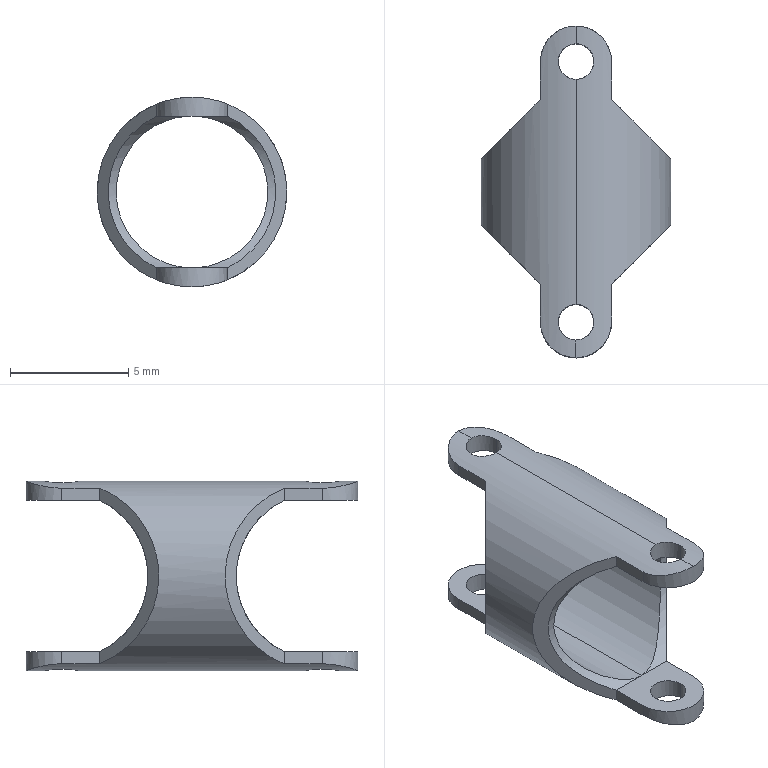Part | SolidWorks | features BaseBody 1, Scale 1 | 1 solid | 36 faces | box 8 x 14 x 8 mm | volume 120.77 mm3 | cylinder 20 | plane 16 | commonest cylinder face diameters 1.5 x8 3 x4 7.068 x4 6.4 x2 8 x2